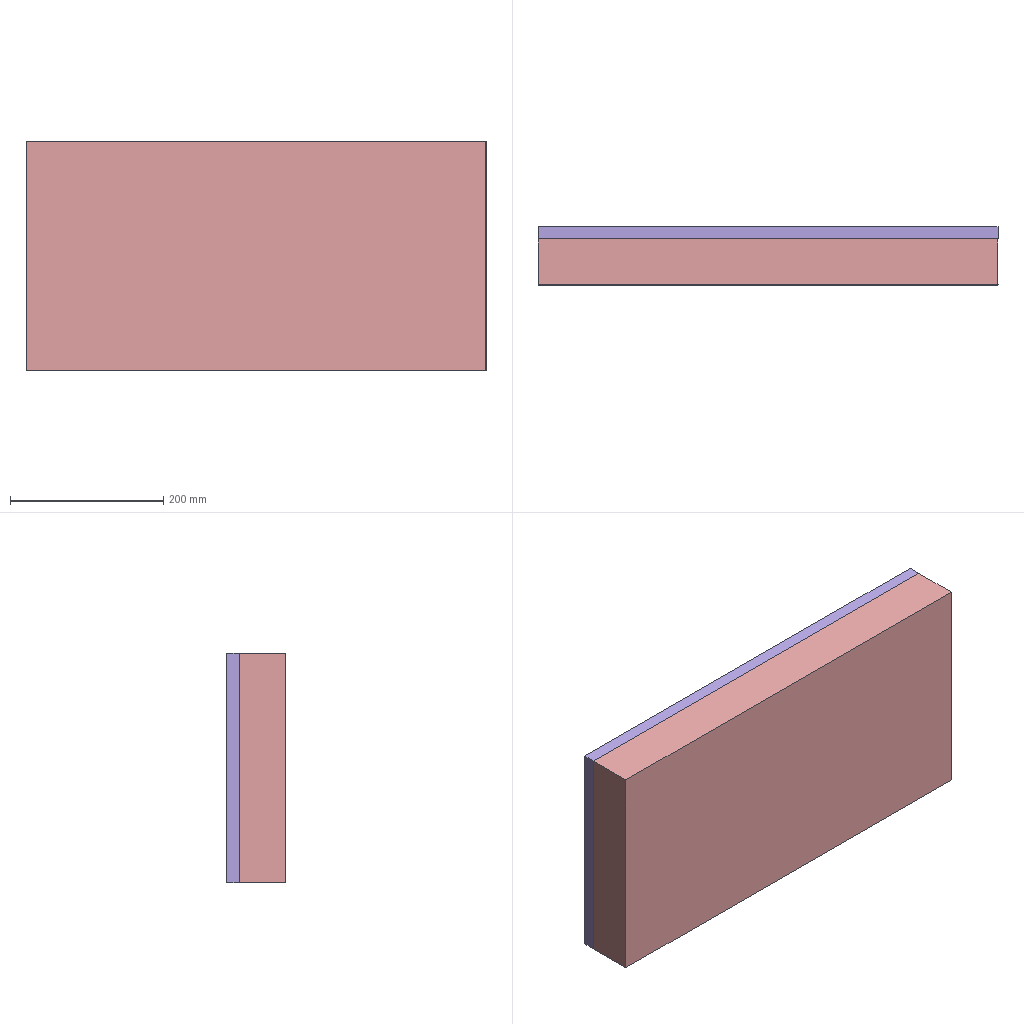Assembly | SolidWorks | 7 different items | 93 placed | box 600 x 76 x 300 mm
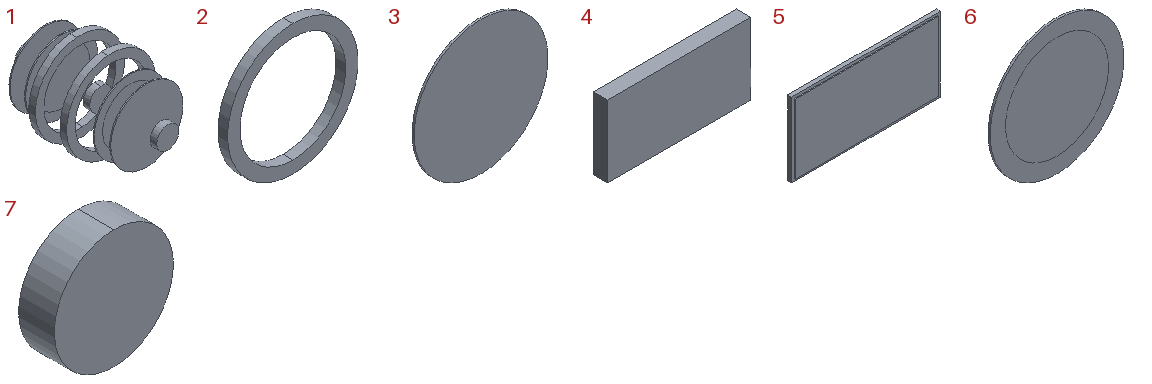Parts list (item | name | quantity | size | volume | features):
1 | (subassembly) | x1 | 80 x 127.615 x 80 mm | 39427 mm3 | -
2 | - | x20 | 80 x 6 x 80 mm | 10249 mm3 | features Extrusion 1
3 | - | x20 | 65 x 1 x 65 mm | 3318 mm3 | features Extrusion 1
4 | - | x1 | 600 x 60 x 300 mm | 7453417 mm3 | features Cut 3, Extrusion 1, LPattern 1
5 | - | x1 | 600 x 20 x 300 mm | 3529600 mm3 | features Extrusion 1, ICE 1
6 | - | x20 | 65 x 1 x 65 mm | 3318 mm3 | features Extrusion 1, ICE 1
7 | - | x30 | 20 x 6 x 20 mm | 1885 mm3 | features Extrusion 1
Mates (type | each side: item.copy, entity, surface, feature):
Coincident | 4.1 plane | assembly plane | 3 times
Concentric | 7.1 face cylinder Boss-Extrude1 | 6.1 face cylinder Boss-Extrude1
Concentric | 7.1 face cylinder Boss-Extrude1 | 7.2 face cylinder Boss-Extrude1
Concentric | 7.1 face cylinder Boss-Extrude1 | 7.3 face cylinder Boss-Extrude1
Concentric | 2.1 face cylinder Boss-Extrude1 | 6.1 face cylinder Boss-Extrude1
Concentric | 2.1 face cylinder Boss-Extrude1 | 3.1 face cylinder Boss-Extrude1
Concentric | 7.2 face cylinder Boss-Extrude1 | 6.2 face cylinder Boss-Extrude1
Concentric | 2.2 face cylinder Boss-Extrude1 | 6.2 face cylinder Boss-Extrude1
Concentric | 2.2 face cylinder Boss-Extrude1 | 3.2 face cylinder Boss-Extrude1
Concentric | 4.1 face cylinder Cut-Extrude1 | 2.2 face cylinder Boss-Extrude1
Coincident | 4.1 face plane Cut-Extrude1 | 7.3 face plane Boss-Extrude1
Concentric | 7.4 face cylinder Boss-Extrude1 | 6.3 face cylinder Boss-Extrude1
Concentric | 7.4 face cylinder Boss-Extrude1 | 7.5 face cylinder Boss-Extrude1
Concentric | 7.4 face cylinder Boss-Extrude1 | 7.6 face cylinder Boss-Extrude1
Concentric | 2.3 face cylinder Boss-Extrude1 | 6.3 face cylinder Boss-Extrude1
Concentric | 2.3 face cylinder Boss-Extrude1 | 3.3 face cylinder Boss-Extrude1
Concentric | 7.5 face cylinder Boss-Extrude1 | 6.4 face cylinder Boss-Extrude1
Concentric | 2.4 face cylinder Boss-Extrude1 | 6.4 face cylinder Boss-Extrude1
Concentric | 2.4 face cylinder Boss-Extrude1 | 3.4 face cylinder Boss-Extrude1
Coincident | 7.1 face plane Boss-Extrude1 | 7.4 face plane Boss-Extrude1
Concentric | 4.1 face cylinder Cut-Extrude1 | 2.3 face cylinder Boss-Extrude1
Coincident | 3.2 face plane Boss-Extrude1 | 7.3 face plane Boss-Extrude1
Coincident | 7.2 face plane Boss-Extrude1 | 6.2 face plane Boss-Extrude2
Coincident | 2.2 face plane Boss-Extrude1 | 6.2 face plane Boss-Extrude1
Coincident | 2.1 face plane Boss-Extrude1 | 2.2 face plane Boss-Extrude1
Coincident | 6.1 face plane Boss-Extrude2 | 7.2 face plane Boss-Extrude1
Coincident | 2.1 face plane Boss-Extrude1 | 3.1 face plane Boss-Extrude1
Coincident | 7.1 face plane Boss-Extrude1 | 3.1 face plane Boss-Extrude1
Coincident | 7.4 face plane Boss-Extrude1 | 3.4 face plane Boss-Extrude1
Coincident | 4.1 face plane Cut-Extrude1 | 7.6 face plane Boss-Extrude1
Coincident | 2.2 face plane Boss-Extrude1 | 2.4 face plane Boss-Extrude1
Coincident | 2.3 face plane Boss-Extrude1 | 2.4 face plane Boss-Extrude1
Coincident | 7.5 face plane Boss-Extrude1 | 6.4 face plane Boss-Extrude2
Coincident | 6.3 face plane Boss-Extrude2 | 7.5 face plane Boss-Extrude1
Coincident | 3.3 face plane Boss-Extrude1 | 6.4 face plane Boss-Extrude2
Coincident | 3.3 face plane Boss-Extrude1 | 7.6 face plane Boss-Extrude1
Coincident | 4.1 face plane Cut-Extrude2 | 5.1 face plane Cut-Extrude1 | 2 times
Coincident | 4.1 face plane Boss-Extrude1 | 5.1 face plane Cut-Extrude1